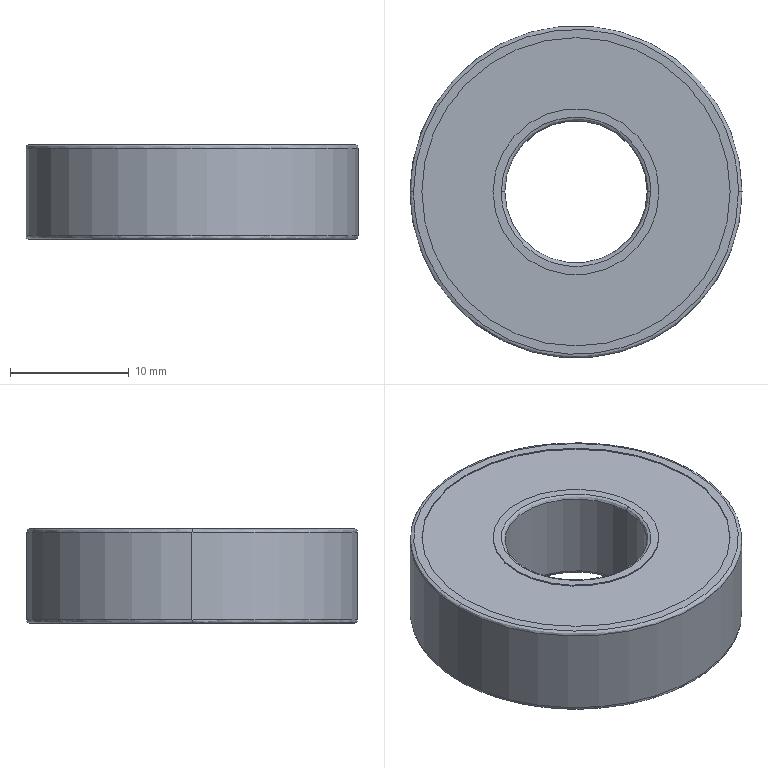Part | SolidWorks | features BaseBody 1 | 1 solid | 26 faces | box 28 x 28 x 8 mm | volume 3942 mm3 | cylinder 12 | spline 8 | plane 6 | commonest cylinder face diameters 14 x4 26 x4 12 x2 28 x2
STEP:
#1=CARTESIAN_POINT('',(-13.7,0.,-8.));
#2=VERTEX_POINT('',#1);
#3=CARTESIAN_POINT('',(13.7,0.,-8.));
#4=VERTEX_POINT('',#3);
#5=CARTESIAN_POINT('',(-13.7,0.,-8.));
#6=CARTESIAN_POINT('',(-13.7,-27.4,-8.));
#7=CARTESIAN_POINT('',(13.7,-27.4,-8.));
#8=CARTESIAN_POINT('',(13.7,0.,-8.));
#9=(BOUNDED_CURVE()B_SPLINE_CURVE(3,(#5,#6,#7,#8),.UNSPECIFIED.,.F.,.F.)B_SPLINE_CURVE_WITH_KNOTS((4,4),(0.,0.5),.UNSPECIFIED.)CURVE()GEOMETRIC_REPRESENTATION_ITEM()RATIONAL_B_SPLINE_CURVE((1.,0.3333,0.3333,1.))REPRESENTATION_ITEM(''));
#10=EDGE_CURVE('',#2,#4,#9,.T.);
#11=ORIENTED_EDGE('',*,*,#10,.T.);
#12=CARTESIAN_POINT('',(14.,0.,-7.7));
#13=VERTEX_POINT('',#12);
#14=CARTESIAN_POINT('',(13.7,0.,-7.7));
#15=DIRECTION('',(0.,-1.,0.));
#16=DIRECTION('',(1.,0.,0.));
#17=AXIS2_PLACEMENT_3D('',#14,#15,#16);
#18=CIRCLE('',#17,0.3);
#19=EDGE_CURVE('',#4,#13,#18,.T.);
#20=ORIENTED_EDGE('',*,*,#19,.T.);
#21=CARTESIAN_POINT('',(-14.,0.,-7.7));
#22=VERTEX_POINT('',#21);
#23=CARTESIAN_POINT('',(0.,0.,-7.7));
#24=DIRECTION('',(0.,0.,1.));
#25=DIRECTION('',(1.,0.,0.));
#26=AXIS2_PLACEMENT_3D('',#23,#24,#25);
#27=CIRCLE('',#26,14.);
#28=EDGE_CURVE('',#22,#13,#27,.T.);
#29=ORIENTED_EDGE('',*,*,#28,.F.);
#30=CARTESIAN_POINT('',(-13.7,0.,-7.7));
#31=DIRECTION('',(0.,1.,0.));
#32=DIRECTION('',(-1.,0.,0.));
#33=AXIS2_PLACEMENT_3D('',#30,#31,#32);
#34=CIRCLE('',#33,0.3);
#35=EDGE_CURVE('',#2,#22,#34,.T.);
#36=ORIENTED_EDGE('',*,*,#35,.F.);
#37=EDGE_LOOP('',(#11,#20,#29,#36));
#38=FACE_OUTER_BOUND('',#37,.T.);
#39=CARTESIAN_POINT('',(13.7,0.,-8.));
#40=CARTESIAN_POINT('',(13.7,-27.4,-8.));
#41=CARTESIAN_POINT('',(-13.7,-27.4,-8.));
#42=CARTESIAN_POINT('',(-13.7,0.,-8.));
#43=CARTESIAN_POINT('',(13.876,0.,-8.));
#44=CARTESIAN_POINT('',(13.876,-27.751,-8.));
#45=CARTESIAN_POINT('',(-13.876,-27.751,-8.));
#46=CARTESIAN_POINT('',(-13.876,0.,-8.));
#47=CARTESIAN_POINT('',(14.,0.,-7.876));
#48=CARTESIAN_POINT('',(14.,-28.,-7.876));
#49=CARTESIAN_POINT('',(-14.,-28.,-7.876));
#50=CARTESIAN_POINT('',(-14.,0.,-7.876));
#51=CARTESIAN_POINT('',(14.,0.,-7.7));
#52=CARTESIAN_POINT('',(14.,-28.,-7.7));
#53=CARTESIAN_POINT('',(-14.,-28.,-7.7));
#54=CARTESIAN_POINT('',(-14.,0.,-7.7));
#55=(BOUNDED_SURFACE()B_SPLINE_SURFACE(3,3,((#39,#40,#41,#42),(#43,#44,#45,#46),(#47,#48,#49,#50),(#51,#52,#53,#54)),.UNSPECIFIED.,.F.,.F.,.F.)B_SPLINE_SURFACE_WITH_KNOTS((4,4),(4,4),(0.,1.),(0.,1.),.UNSPECIFIED.)GEOMETRIC_REPRESENTATION_ITEM()RATIONAL_B_SPLINE_SURFACE(((1.,0.3333,0.3333,1.),(0.8047,0.2682,0.2682,0.8047),(0.8047,0.2682,0.2682,0.8047),(1.,0.3333,0.3333,1.)))REPRESENTATION_ITEM('')SURFACE());
#56=ADVANCED_FACE('',(#38),#55,.T.);
#57=CARTESIAN_POINT('',(14.,0.,-0.3));
#58=VERTEX_POINT('',#57);
#59=CARTESIAN_POINT('',(-14.,0.,-0.3));
#60=VERTEX_POINT('',#59);
#61=CARTESIAN_POINT('',(0.,0.,-0.3));
#62=DIRECTION('',(0.,0.,-1.));
#63=DIRECTION('',(1.,0.,0.));
#64=AXIS2_PLACEMENT_3D('',#61,#62,#63);
#65=CIRCLE('',#64,14.);
#66=EDGE_CURVE('',#58,#60,#65,.T.);
#67=ORIENTED_EDGE('',*,*,#66,.F.);
#68=CARTESIAN_POINT('',(13.7,0.,0.));
#69=VERTEX_POINT('',#68);
#70=CARTESIAN_POINT('',(13.7,0.,-0.3));
#71=DIRECTION('',(0.,-1.,0.));
#72=DIRECTION('',(1.,0.,0.));
#73=AXIS2_PLACEMENT_3D('',#70,#71,#72);
#74=CIRCLE('',#73,0.3);
#75=EDGE_CURVE('',#58,#69,#74,.T.);
#76=ORIENTED_EDGE('',*,*,#75,.T.);
#77=CARTESIAN_POINT('',(-13.7,0.,0.));
#78=VERTEX_POINT('',#77);
#79=CARTESIAN_POINT('',(13.7,0.,0.));
#80=CARTESIAN_POINT('',(13.7,-27.4,0.));
#81=CARTESIAN_POINT('',(-13.7,-27.4,0.));
#82=CARTESIAN_POINT('',(-13.7,0.,0.));
#83=(BOUNDED_CURVE()B_SPLINE_CURVE(3,(#79,#80,#81,#82),.UNSPECIFIED.,.F.,.F.)B_SPLINE_CURVE_WITH_KNOTS((4,4),(0.5,1.),.UNSPECIFIED.)CURVE()GEOMETRIC_REPRESENTATION_ITEM()RATIONAL_B_SPLINE_CURVE((1.,0.3333,0.3333,1.))REPRESENTATION_ITEM(''));
#84=EDGE_CURVE('',#69,#78,#83,.T.);
#85=ORIENTED_EDGE('',*,*,#84,.T.);
#86=CARTESIAN_POINT('',(-13.7,0.,-0.3));
#87=DIRECTION('',(0.,1.,0.));
#88=DIRECTION('',(-1.,0.,0.));
#89=AXIS2_PLACEMENT_3D('',#86,#87,#88);
#90=CIRCLE('',#89,0.3);
#91=EDGE_CURVE('',#60,#78,#90,.T.);
#92=ORIENTED_EDGE('',*,*,#91,.F.);
#93=EDGE_LOOP('',(#67,#76,#85,#92));
#94=FACE_OUTER_BOUND('',#93,.T.);
#95=CARTESIAN_POINT('',(14.,0.,-0.3));
#96=CARTESIAN_POINT('',(14.,-28.,-0.3));
#97=CARTESIAN_POINT('',(-14.,-28.,-0.3));
#98=CARTESIAN_POINT('',(-14.,0.,-0.3));
#99=CARTESIAN_POINT('',(14.,0.,-0.1243));
#100=CARTESIAN_POINT('',(14.,-28.,-0.1243));
#101=CARTESIAN_POINT('',(-14.,-28.,-0.1243));
#102=CARTESIAN_POINT('',(-14.,0.,-0.1243));
#103=CARTESIAN_POINT('',(13.876,0.,0.));
#104=CARTESIAN_POINT('',(13.876,-27.751,0.));
#105=CARTESIAN_POINT('',(-13.876,-27.751,0.));
#106=CARTESIAN_POINT('',(-13.876,0.,0.));
#107=CARTESIAN_POINT('',(13.7,0.,0.));
#108=CARTESIAN_POINT('',(13.7,-27.4,0.));
#109=CARTESIAN_POINT('',(-13.7,-27.4,0.));
#110=CARTESIAN_POINT('',(-13.7,0.,0.));
#111=(BOUNDED_SURFACE()B_SPLINE_SURFACE(3,3,((#95,#96,#97,#98),(#99,#100,#101,#102),(#103,#104,#105,#106),(#107,#108,#109,#110)),.UNSPECIFIED.,.F.,.F.,.F.)B_SPLINE_SURFACE_WITH_KNOTS((4,4),(4,4),(0.,1.),(0.,1.),.UNSPECIFIED.)GEOMETRIC_REPRESENTATION_ITEM()RATIONAL_B_SPLINE_SURFACE(((1.,0.3333,0.3333,1.),(0.8047,0.2682,0.2682,0.8047),(0.8047,0.2682,0.2682,0.8047),(1.,0.3333,0.3333,1.)))REPRESENTATION_ITEM('')SURFACE());
#112=ADVANCED_FACE('',(#94),#111,.T.);
#113=CARTESIAN_POINT('',(-6.,0.,-7.7));
#114=VERTEX_POINT('',#113);
#115=CARTESIAN_POINT('',(6.,0.,-7.7));
#116=VERTEX_POINT('',#115);
#117=CARTESIAN_POINT('',(0.,0.,-7.7));
#118=DIRECTION('',(0.,0.,1.));
#119=DIRECTION('',(-1.,0.,0.));
#120=AXIS2_PLACEMENT_3D('',#117,#118,#119);
#121=CIRCLE('',#120,6.);
#122=EDGE_CURVE('',#114,#116,#121,.T.);
#123=ORIENTED_EDGE('',*,*,#122,.T.);
#124=CARTESIAN_POINT('',(6.3,0.,-8.));
#125=VERTEX_POINT('',#124);
#126=CARTESIAN_POINT('',(6.3,0.,-7.7));
#127=DIRECTION('',(0.,-1.,0.));
#128=DIRECTION('',(1.,0.,0.));
#129=AXIS2_PLACEMENT_3D('',#126,#127,#128);
#130=CIRCLE('',#129,0.3);
#131=EDGE_CURVE('',#116,#125,#130,.T.);
#132=ORIENTED_EDGE('',*,*,#131,.T.);
#133=CARTESIAN_POINT('',(-6.3,0.,-8.));
#134=VERTEX_POINT('',#133);
#135=CARTESIAN_POINT('',(-6.3,0.,-8.));
#136=CARTESIAN_POINT('',(-6.3,-0.1926,-8.));
#137=CARTESIAN_POINT('',(-6.287,-0.4803,-8.));
#138=CARTESIAN_POINT('',(-6.249,-0.814,-8.));
#139=CARTESIAN_POINT('',(-6.224,-0.9804,-8.));
#140=CARTESIAN_POINT('',(-6.212,-1.052,-8.));
#141=CARTESIAN_POINT('',(-6.203,-1.099,-8.));
#142=CARTESIAN_POINT('',(-6.199,-1.121,-8.));
#143=CARTESIAN_POINT('',(-6.158,-1.347,-8.));
#144=CARTESIAN_POINT('',(-6.088,-1.644,-8.));
#145=CARTESIAN_POINT('',(-5.981,-1.984,-8.));
#146=CARTESIAN_POINT('',(-5.93,-2.128,-8.));
#147=CARTESIAN_POINT('',(-5.895,-2.224,-8.));
#148=CARTESIAN_POINT('',(-5.877,-2.27,-8.));
#149=CARTESIAN_POINT('',(-5.779,-2.517,-8.));
#150=CARTESIAN_POINT('',(-5.648,-2.806,-8.));
#151=CARTESIAN_POINT('',(-5.494,-3.085,-8.));
#152=CARTESIAN_POINT('',(-5.387,-3.268,-8.));
#153=CARTESIAN_POINT('',(-5.333,-3.356,-8.));
#154=CARTESIAN_POINT('',(-5.035,-3.811,-8.));
#155=CARTESIAN_POINT('',(-4.762,-4.147,-8.));
#156=CARTESIAN_POINT('',(-4.301,-4.608,-8.));
#157=CARTESIAN_POINT('',(-4.06,-4.826,-8.));
#158=CARTESIAN_POINT('',(-3.76,-5.057,-8.));
#159=CARTESIAN_POINT('',(-3.627,-5.151,-8.));
#160=CARTESIAN_POINT('',(-3.538,-5.213,-8.));
#161=CARTESIAN_POINT('',(-3.492,-5.244,-8.));
#162=CARTESIAN_POINT('',(-3.269,-5.389,-8.));
#163=CARTESIAN_POINT('',(-2.995,-5.55,-8.));
#164=CARTESIAN_POINT('',(-2.661,-5.712,-8.));
#165=CARTESIAN_POINT('',(-2.516,-5.776,-8.));
#166=CARTESIAN_POINT('',(-2.418,-5.818,-8.));
#167=CARTESIAN_POINT('',(-2.366,-5.839,-8.));
#168=CARTESIAN_POINT('',(-2.129,-5.933,-8.));
#169=CARTESIAN_POINT('',(-1.84,-6.031,-8.));
#170=CARTESIAN_POINT('',(-1.496,-6.121,-8.));
#171=CARTESIAN_POINT('',(-1.322,-6.16,-8.));
#172=CARTESIAN_POINT('',(-1.247,-6.175,-8.));
#173=CARTESIAN_POINT('',(-1.197,-6.185,-8.));
#174=CARTESIAN_POINT('',(-1.17,-6.19,-8.));
#175=CARTESIAN_POINT('',(-0.7678,-6.265,-8.));
#176=CARTESIAN_POINT('',(-0.385,-6.3,-8.));
#177=CARTESIAN_POINT('',(0.1925,-6.3,-8.));
#178=CARTESIAN_POINT('',(0.4802,-6.287,-8.));
#179=CARTESIAN_POINT('',(0.8139,-6.249,-8.));
#180=CARTESIAN_POINT('',(0.9803,-6.224,-8.));
#181=CARTESIAN_POINT('',(1.051,-6.212,-8.));
#182=CARTESIAN_POINT('',(1.099,-6.203,-8.));
#183=CARTESIAN_POINT('',(1.121,-6.199,-8.));
#184=CARTESIAN_POINT('',(1.347,-6.158,-8.));
#185=CARTESIAN_POINT('',(1.644,-6.088,-8.));
#186=CARTESIAN_POINT('',(1.984,-5.981,-8.));
#187=CARTESIAN_POINT('',(2.128,-5.93,-8.));
#188=CARTESIAN_POINT('',(2.224,-5.895,-8.));
#189=CARTESIAN_POINT('',(2.27,-5.877,-8.));
#190=CARTESIAN_POINT('',(2.517,-5.779,-8.));
#191=CARTESIAN_POINT('',(2.806,-5.648,-8.));
#192=CARTESIAN_POINT('',(3.085,-5.494,-8.));
#193=CARTESIAN_POINT('',(3.268,-5.387,-8.));
#194=CARTESIAN_POINT('',(3.356,-5.333,-8.));
#195=CARTESIAN_POINT('',(3.811,-5.035,-8.));
#196=CARTESIAN_POINT('',(4.147,-4.762,-8.));
#197=CARTESIAN_POINT('',(4.608,-4.301,-8.));
#198=CARTESIAN_POINT('',(4.826,-4.06,-8.));
#199=CARTESIAN_POINT('',(5.057,-3.76,-8.));
#200=CARTESIAN_POINT('',(5.151,-3.627,-8.));
#201=CARTESIAN_POINT('',(5.213,-3.538,-8.));
#202=CARTESIAN_POINT('',(5.244,-3.492,-8.));
#203=CARTESIAN_POINT('',(5.389,-3.269,-8.));
#204=CARTESIAN_POINT('',(5.55,-2.995,-8.));
#205=CARTESIAN_POINT('',(5.712,-2.661,-8.));
#206=CARTESIAN_POINT('',(5.776,-2.516,-8.));
#207=CARTESIAN_POINT('',(5.818,-2.418,-8.));
#208=CARTESIAN_POINT('',(5.839,-2.366,-8.));
#209=CARTESIAN_POINT('',(5.933,-2.129,-8.));
#210=CARTESIAN_POINT('',(6.031,-1.84,-8.));
#211=CARTESIAN_POINT('',(6.121,-1.496,-8.));
#212=CARTESIAN_POINT('',(6.16,-1.322,-8.));
#213=CARTESIAN_POINT('',(6.175,-1.247,-8.));
#214=CARTESIAN_POINT('',(6.185,-1.197,-8.));
#215=CARTESIAN_POINT('',(6.19,-1.17,-8.));
#216=CARTESIAN_POINT('',(6.265,-0.7678,-8.));
#217=CARTESIAN_POINT('',(6.3,-0.385,-8.));
#218=CARTESIAN_POINT('',(6.3,0.,-8.));
#219=B_SPLINE_CURVE_WITH_KNOTS('',3,(#135,#136,#137,#138,#139,#140,#141,#142,#143,#144,#145,#146,#147,#148,#149,#150,#151,#152,#153,#154,#155,#156,#157,#158,#159,#160,#161,#162,#163,#164,#165,#166,#167,#168,#169,#170,#171,#172,#173,#174,#175,#176,#177,#178,#179,#180,#181,#182,#183,#184,#185,#186,#187,#188,#189,#190,#191,#192,#193,#194,#195,#196,#197,#198,#199,#200,#201,#202,#203,#204,#205,#206,#207,#208,#209,#210,#211,#212,#213,#214,#215,#216,#217,#218),.UNSPECIFIED.,.F.,.F.,(4,1,1,1,2,2,1,1,2,2,1,2,2,2,1,1,2,2,1,1,2,2,1,1,1,2,2,2,1,1,1,2,2,1,1,2,2,1,2,2,2,1,1,2,2,1,1,2,2,1,1,1,2,2,4),(0.,0.01563,0.02344,0.02734,0.0293,0.03125,0.04688,0.05469,0.05859,0.0625,0.07813,0.08594,0.09375,0.125,0.1406,0.1484,0.1523,0.1563,0.1719,0.1797,0.1836,0.1875,0.2031,0.2109,0.2148,0.2168,0.2188,0.25,0.2656,0.2734,0.2773,0.2793,0.2813,0.2969,0.3047,0.3086,0.3125,0.3281,0.3359,0.3438,0.375,0.3906,0.3984,0.4023,0.4063,0.4219,0.4297,0.4336,0.4375,0.4531,0.4609,0.4648,0.4668,0.4688,0.5),.UNSPECIFIED.);
#220=EDGE_CURVE('',#134,#125,#219,.T.);
#221=ORIENTED_EDGE('',*,*,#220,.F.);
#222=CARTESIAN_POINT('',(-6.3,0.,-7.7));
#223=DIRECTION('',(0.,1.,0.));
#224=DIRECTION('',(-1.,0.,0.));
#225=AXIS2_PLACEMENT_3D('',#222,#223,#224);
#226=CIRCLE('',#225,0.3);
#227=EDGE_CURVE('',#114,#134,#226,.T.);
#228=ORIENTED_EDGE('',*,*,#227,.F.);
#229=EDGE_LOOP('',(#123,#132,#221,#228));
#230=FACE_OUTER_BOUND('',#229,.T.);
#231=CARTESIAN_POINT('',(6.,0.,-7.7));
#232=CARTESIAN_POINT('',(6.,-12.,-7.7));
#233=CARTESIAN_POINT('',(-6.,-12.,-7.7));
#234=CARTESIAN_POINT('',(-6.,0.,-7.7));
#235=CARTESIAN_POINT('',(6.,0.,-7.876));
#236=CARTESIAN_POINT('',(6.,-12.,-7.876));
#237=CARTESIAN_POINT('',(-6.,-12.,-7.876));
#238=CARTESIAN_POINT('',(-6.,0.,-7.876));
#239=CARTESIAN_POINT('',(6.124,0.,-8.));
#240=CARTESIAN_POINT('',(6.124,-12.249,-8.));
#241=CARTESIAN_POINT('',(-6.124,-12.249,-8.));
#242=CARTESIAN_POINT('',(-6.124,0.,-8.));
#243=CARTESIAN_POINT('',(6.3,0.,-8.));
#244=CARTESIAN_POINT('',(6.3,-12.6,-8.));
#245=CARTESIAN_POINT('',(-6.3,-12.6,-8.));
#246=CARTESIAN_POINT('',(-6.3,0.,-8.));
#247=(BOUNDED_SURFACE()B_SPLINE_SURFACE(3,3,((#231,#232,#233,#234),(#235,#236,#237,#238),(#239,#240,#241,#242),(#243,#244,#245,#246)),.UNSPECIFIED.,.F.,.F.,.F.)B_SPLINE_SURFACE_WITH_KNOTS((4,4),(4,4),(0.,1.),(0.,1.),.UNSPECIFIED.)GEOMETRIC_REPRESENTATION_ITEM()RATIONAL_B_SPLINE_SURFACE(((1.,0.3333,0.3333,1.),(0.8047,0.2682,0.2682,0.8047),(0.8047,0.2682,0.2682,0.8047),(1.,0.3333,0.3333,1.)))REPRESENTATION_ITEM('')SURFACE());
#248=ADVANCED_FACE('',(#230),#247,.T.);
#249=CARTESIAN_POINT('',(6.3,0.,0.));
#250=VERTEX_POINT('',#249);
#251=CARTESIAN_POINT('',(-6.3,0.,0.));
#252=VERTEX_POINT('',#251);
#253=CARTESIAN_POINT('',(6.3,0.,0.));
#254=CARTESIAN_POINT('',(6.3,-0.1925,0.));
#255=CARTESIAN_POINT('',(6.287,-0.4802,0.));
#256=CARTESIAN_POINT('',(6.249,-0.8139,0.));
#257=CARTESIAN_POINT('',(6.224,-0.9803,0.));
#258=CARTESIAN_POINT('',(6.212,-1.051,0.));
#259=CARTESIAN_POINT('',(6.203,-1.099,0.));
#260=CARTESIAN_POINT('',(6.199,-1.121,0.));
#261=CARTESIAN_POINT('',(6.158,-1.347,0.));
#262=CARTESIAN_POINT('',(6.088,-1.644,0.));
#263=CARTESIAN_POINT('',(5.981,-1.984,0.));
#264=CARTESIAN_POINT('',(5.93,-2.128,0.));
#265=CARTESIAN_POINT('',(5.895,-2.224,0.));
#266=CARTESIAN_POINT('',(5.877,-2.27,0.));
#267=CARTESIAN_POINT('',(5.779,-2.517,0.));
#268=CARTESIAN_POINT('',(5.648,-2.806,0.));
#269=CARTESIAN_POINT('',(5.494,-3.085,0.));
#270=CARTESIAN_POINT('',(5.387,-3.268,0.));
#271=CARTESIAN_POINT('',(5.333,-3.356,0.));
#272=CARTESIAN_POINT('',(5.035,-3.811,0.));
#273=CARTESIAN_POINT('',(4.762,-4.147,0.));
#274=CARTESIAN_POINT('',(4.301,-4.608,0.));
#275=CARTESIAN_POINT('',(4.06,-4.826,0.));
#276=CARTESIAN_POINT('',(3.76,-5.057,0.));
#277=CARTESIAN_POINT('',(3.627,-5.151,0.));
#278=CARTESIAN_POINT('',(3.538,-5.213,0.));
#279=CARTESIAN_POINT('',(3.492,-5.244,0.));
#280=CARTESIAN_POINT('',(3.269,-5.389,0.));
#281=CARTESIAN_POINT('',(2.995,-5.55,0.));
#282=CARTESIAN_POINT('',(2.661,-5.712,0.));
#283=CARTESIAN_POINT('',(2.516,-5.776,0.));
#284=CARTESIAN_POINT('',(2.418,-5.818,0.));
#285=CARTESIAN_POINT('',(2.366,-5.839,0.));
#286=CARTESIAN_POINT('',(2.129,-5.933,0.));
#287=CARTESIAN_POINT('',(1.84,-6.031,0.));
#288=CARTESIAN_POINT('',(1.496,-6.121,0.));
#289=CARTESIAN_POINT('',(1.322,-6.16,0.));
#290=CARTESIAN_POINT('',(1.247,-6.175,0.));
#291=CARTESIAN_POINT('',(1.197,-6.185,0.));
#292=CARTESIAN_POINT('',(1.17,-6.19,0.));
#293=CARTESIAN_POINT('',(0.7678,-6.265,0.));
#294=CARTESIAN_POINT('',(0.385,-6.3,0.));
#295=CARTESIAN_POINT('',(-0.1925,-6.3,0.));
#296=CARTESIAN_POINT('',(-0.4802,-6.287,0.));
#297=CARTESIAN_POINT('',(-0.8139,-6.249,0.));
#298=CARTESIAN_POINT('',(-0.9803,-6.224,0.));
#299=CARTESIAN_POINT('',(-1.051,-6.212,0.));
#300=CARTESIAN_POINT('',(-1.099,-6.203,0.));
#301=CARTESIAN_POINT('',(-1.121,-6.199,0.));
#302=CARTESIAN_POINT('',(-1.347,-6.158,0.));
#303=CARTESIAN_POINT('',(-1.644,-6.088,0.));
#304=CARTESIAN_POINT('',(-1.984,-5.981,0.));
#305=CARTESIAN_POINT('',(-2.128,-5.93,0.));
#306=CARTESIAN_POINT('',(-2.224,-5.895,0.));
#307=CARTESIAN_POINT('',(-2.27,-5.877,0.));
#308=CARTESIAN_POINT('',(-2.517,-5.779,0.));
#309=CARTESIAN_POINT('',(-2.806,-5.648,0.));
#310=CARTESIAN_POINT('',(-3.085,-5.494,0.));
#311=CARTESIAN_POINT('',(-3.268,-5.387,0.));
#312=CARTESIAN_POINT('',(-3.356,-5.333,0.));
#313=CARTESIAN_POINT('',(-3.811,-5.035,0.));
#314=CARTESIAN_POINT('',(-4.147,-4.762,0.));
#315=CARTESIAN_POINT('',(-4.608,-4.301,0.));
#316=CARTESIAN_POINT('',(-4.826,-4.06,0.));
#317=CARTESIAN_POINT('',(-5.057,-3.76,0.));
#318=CARTESIAN_POINT('',(-5.151,-3.627,0.));
#319=CARTESIAN_POINT('',(-5.213,-3.538,0.));
#320=CARTESIAN_POINT('',(-5.244,-3.492,0.));
#321=CARTESIAN_POINT('',(-5.389,-3.269,0.));
#322=CARTESIAN_POINT('',(-5.55,-2.995,0.));
#323=CARTESIAN_POINT('',(-5.712,-2.661,0.));
#324=CARTESIAN_POINT('',(-5.776,-2.516,0.));
#325=CARTESIAN_POINT('',(-5.818,-2.418,0.));
#326=CARTESIAN_POINT('',(-5.839,-2.366,0.));
#327=CARTESIAN_POINT('',(-5.933,-2.129,0.));
#328=CARTESIAN_POINT('',(-6.031,-1.84,0.));
#329=CARTESIAN_POINT('',(-6.121,-1.496,0.));
#330=CARTESIAN_POINT('',(-6.16,-1.322,0.));
#331=CARTESIAN_POINT('',(-6.175,-1.247,0.));
#332=CARTESIAN_POINT('',(-6.185,-1.197,0.));
#333=CARTESIAN_POINT('',(-6.19,-1.17,0.));
#334=CARTESIAN_POINT('',(-6.265,-0.7676,0.));
#335=CARTESIAN_POINT('',(-6.3,-0.3855,0.));
#336=CARTESIAN_POINT('',(-6.3,0.,0.));
#337=B_SPLINE_CURVE_WITH_KNOTS('',3,(#253,#254,#255,#256,#257,#258,#259,#260,#261,#262,#263,#264,#265,#266,#267,#268,#269,#270,#271,#272,#273,#274,#275,#276,#277,#278,#279,#280,#281,#282,#283,#284,#285,#286,#287,#288,#289,#290,#291,#292,#293,#294,#295,#296,#297,#298,#299,#300,#301,#302,#303,#304,#305,#306,#307,#308,#309,#310,#311,#312,#313,#314,#315,#316,#317,#318,#319,#320,#321,#322,#323,#324,#325,#326,#327,#328,#329,#330,#331,#332,#333,#334,#335,#336),.UNSPECIFIED.,.F.,.F.,(4,1,1,1,2,2,1,1,2,2,1,2,2,2,1,1,2,2,1,1,2,2,1,1,1,2,2,2,1,1,1,2,2,1,1,2,2,1,2,2,2,1,1,2,2,1,1,2,2,1,1,1,2,2,4),(0.5,0.5156,0.5234,0.5273,0.5293,0.5313,0.5469,0.5547,0.5586,0.5625,0.5781,0.5859,0.5938,0.625,0.6406,0.6484,0.6523,0.6563,0.6719,0.6797,0.6836,0.6875,0.7031,0.7109,0.7148,0.7168,0.7188,0.75,0.7656,0.7734,0.7773,0.7793,0.7813,0.7969,0.8047,0.8086,0.8125,0.8281,0.8359,0.8438,0.875,0.8906,0.8984,0.9023,0.9063,0.9219,0.9297,0.9336,0.9375,0.9531,0.9609,0.9648,0.9668,0.9688,1.),.UNSPECIFIED.);
#338=EDGE_CURVE('',#250,#252,#337,.T.);
#339=ORIENTED_EDGE('',*,*,#338,.F.);
#340=CARTESIAN_POINT('',(6.,0.,-0.3));
#341=VERTEX_POINT('',#340);
#342=CARTESIAN_POINT('',(6.3,0.,-0.3));
#343=DIRECTION('',(0.,-1.,0.));
#344=DIRECTION('',(1.,0.,0.));
#345=AXIS2_PLACEMENT_3D('',#342,#343,#344);
#346=CIRCLE('',#345,0.3);
#347=EDGE_CURVE('',#250,#341,#346,.T.);
#348=ORIENTED_EDGE('',*,*,#347,.T.);
#349=CARTESIAN_POINT('',(-6.,0.,-0.3));
#350=VERTEX_POINT('',#349);
#351=CARTESIAN_POINT('',(0.,0.,-0.3));
#352=DIRECTION('',(0.,0.,-1.));
#353=DIRECTION('',(-1.,0.,0.));
#354=AXIS2_PLACEMENT_3D('',#351,#352,#353);
#355=CIRCLE('',#354,6.);
#356=EDGE_CURVE('',#341,#350,#355,.T.);
#357=ORIENTED_EDGE('',*,*,#356,.T.);
#358=CARTESIAN_POINT('',(-6.3,0.,-0.3));
#359=DIRECTION('',(0.,1.,0.));
#360=DIRECTION('',(-1.,0.,0.));
#361=AXIS2_PLACEMENT_3D('',#358,#359,#360);
#362=CIRCLE('',#361,0.3);
#363=EDGE_CURVE('',#252,#350,#362,.T.);
#364=ORIENTED_EDGE('',*,*,#363,.F.);
#365=EDGE_LOOP('',(#339,#348,#357,#364));
#366=FACE_OUTER_BOUND('',#365,.T.);
#367=CARTESIAN_POINT('',(6.3,0.,0.));
#368=CARTESIAN_POINT('',(6.3,-12.6,0.));
#369=CARTESIAN_POINT('',(-6.3,-12.6,0.));
#370=CARTESIAN_POINT('',(-6.3,0.,0.));
#371=CARTESIAN_POINT('',(6.124,0.,0.));
#372=CARTESIAN_POINT('',(6.124,-12.249,0.));
#373=CARTESIAN_POINT('',(-6.124,-12.249,0.));
#374=CARTESIAN_POINT('',(-6.124,0.,0.));
#375=CARTESIAN_POINT('',(6.,0.,-0.1243));
#376=CARTESIAN_POINT('',(6.,-12.,-0.1243));
#377=CARTESIAN_POINT('',(-6.,-12.,-0.1243));
#378=CARTESIAN_POINT('',(-6.,0.,-0.1243));
#379=CARTESIAN_POINT('',(6.,0.,-0.3));
#380=CARTESIAN_POINT('',(6.,-12.,-0.3));
#381=CARTESIAN_POINT('',(-6.,-12.,-0.3));
#382=CARTESIAN_POINT('',(-6.,0.,-0.3));
#383=(BOUNDED_SURFACE()B_SPLINE_SURFACE(3,3,((#367,#368,#369,#370),(#371,#372,#373,#374),(#375,#376,#377,#378),(#379,#380,#381,#382)),.UNSPECIFIED.,.F.,.F.,.F.)B_SPLINE_SURFACE_WITH_KNOTS((4,4),(4,4),(0.,1.),(0.,1.),.UNSPECIFIED.)GEOMETRIC_REPRESENTATION_ITEM()RATIONAL_B_SPLINE_SURFACE(((1.,0.3333,0.3333,1.),(0.8047,0.2682,0.2682,0.8047),(0.8047,0.2682,0.2682,0.8047),(1.,0.3333,0.3333,1.)))REPRESENTATION_ITEM('')SURFACE());
#384=ADVANCED_FACE('',(#366),#383,.T.);
#385=CARTESIAN_POINT('',(0.,0.,-7.7));
#386=DIRECTION('',(0.,0.,1.));
#387=DIRECTION('',(1.,0.,0.));
#388=AXIS2_PLACEMENT_3D('',#385,#386,#387);
#389=CIRCLE('',#388,14.);
#390=EDGE_CURVE('',#13,#22,#389,.T.);
#391=ORIENTED_EDGE('',*,*,#390,.T.);
#392=CARTESIAN_POINT('',(-14.,0.,-8.));
#393=DIRECTION('',(0.,0.,1.));
#394=VECTOR('',#393,1000.);
#395=LINE('',#392,#394);
#396=EDGE_CURVE('',#22,#60,#395,.T.);
#397=ORIENTED_EDGE('',*,*,#396,.T.);
#398=CARTESIAN_POINT('',(0.,0.,-0.3));
#399=DIRECTION('',(0.,0.,-1.));
#400=DIRECTION('',(1.,0.,0.));
#401=AXIS2_PLACEMENT_3D('',#398,#399,#400);
#402=CIRCLE('',#401,14.);
#403=EDGE_CURVE('',#60,#58,#402,.T.);
#404=ORIENTED_EDGE('',*,*,#403,.T.);
#405=CARTESIAN_POINT('',(14.,0.,-8.));
#406=DIRECTION('',(0.,0.,1.));
#407=VECTOR('',#406,1000.);
#408=LINE('',#405,#407);
#409=EDGE_CURVE('',#13,#58,#408,.T.);
#410=ORIENTED_EDGE('',*,*,#409,.F.);
#411=EDGE_LOOP('',(#391,#397,#404,#410));
#412=FACE_OUTER_BOUND('',#411,.T.);
#413=CARTESIAN_POINT('',(0.,0.,-8.));
#414=DIRECTION('',(0.,0.,1.));
#415=DIRECTION('',(1.,0.,0.));
#416=AXIS2_PLACEMENT_3D('',#413,#414,#415);
#417=CYLINDRICAL_SURFACE('',#416,14.);
#418=ADVANCED_FACE('',(#412),#417,.T.);
#419=CARTESIAN_POINT('',(-13.,0.,-8.));
#420=VERTEX_POINT('',#419);
#421=CARTESIAN_POINT('',(13.,0.,-8.));
#422=VERTEX_POINT('',#421);
#423=CARTESIAN_POINT('',(0.,0.,-8.));
#424=DIRECTION('',(0.,0.,1.));
#425=DIRECTION('',(1.,0.,0.));
#426=AXIS2_PLACEMENT_3D('',#423,#424,#425);
#427=CIRCLE('',#426,13.);
#428=EDGE_CURVE('',#420,#422,#427,.T.);
#429=ORIENTED_EDGE('',*,*,#428,.F.);
#430=CARTESIAN_POINT('',(-13.,0.,-7.9));
#431=VERTEX_POINT('',#430);
#432=CARTESIAN_POINT('',(-13.,0.,-8.));
#433=DIRECTION('',(0.,0.,1.));
#434=VECTOR('',#433,1000.);
#435=LINE('',#432,#434);
#436=EDGE_CURVE('',#420,#431,#435,.T.);
#437=ORIENTED_EDGE('',*,*,#436,.T.);
#438=CARTESIAN_POINT('',(13.,0.,-7.9));
#439=VERTEX_POINT('',#438);
#440=CARTESIAN_POINT('',(0.,0.,-7.9));
#441=DIRECTION('',(0.,0.,-1.));
#442=DIRECTION('',(1.,0.,0.));
#443=AXIS2_PLACEMENT_3D('',#440,#441,#442);
#444=CIRCLE('',#443,13.);
#445=EDGE_CURVE('',#439,#431,#444,.T.);
#446=ORIENTED_EDGE('',*,*,#445,.F.);
#447=CARTESIAN_POINT('',(13.,0.,-8.));
#448=DIRECTION('',(0.,0.,1.));
#449=VECTOR('',#448,1000.);
#450=LINE('',#447,#449);
#451=EDGE_CURVE('',#422,#439,#450,.T.);
#452=ORIENTED_EDGE('',*,*,#451,.F.);
#453=EDGE_LOOP('',(#429,#437,#446,#452));
#454=FACE_OUTER_BOUND('',#453,.T.);
#455=CARTESIAN_POINT('',(0.,0.,-8.));
#456=DIRECTION('',(0.,0.,1.));
#457=DIRECTION('',(1.,0.,0.));
#458=AXIS2_PLACEMENT_3D('',#455,#456,#457);
#459=CYLINDRICAL_SURFACE('',#458,13.);
#460=ADVANCED_FACE('',(#454),#459,.F.);
#461=CARTESIAN_POINT('',(-13.,0.,-0.1));
#462=VERTEX_POINT('',#461);
#463=CARTESIAN_POINT('',(13.,0.,-0.1));
#464=VERTEX_POINT('',#463);
#465=CARTESIAN_POINT('',(0.,0.,-0.1));
#466=DIRECTION('',(0.,0.,1.));
#467=DIRECTION('',(1.,0.,0.));
#468=AXIS2_PLACEMENT_3D('',#465,#466,#467);
#469=CIRCLE('',#468,13.);
#470=EDGE_CURVE('',#462,#464,#469,.T.);
#471=ORIENTED_EDGE('',*,*,#470,.F.);
#472=CARTESIAN_POINT('',(-13.,0.,0.));
#473=VERTEX_POINT('',#472);
#474=CARTESIAN_POINT('',(-13.,0.,-8.));
#475=DIRECTION('',(0.,0.,1.));
#476=VECTOR('',#475,1000.);
#477=LINE('',#474,#476);
#478=EDGE_CURVE('',#462,#473,#477,.T.);
#479=ORIENTED_EDGE('',*,*,#478,.T.);
#480=CARTESIAN_POINT('',(13.,0.,0.));
#481=VERTEX_POINT('',#480);
#482=CARTESIAN_POINT('',(0.,0.,0.));
#483=DIRECTION('',(0.,0.,-1.));
#484=DIRECTION('',(1.,0.,0.));
#485=AXIS2_PLACEMENT_3D('',#482,#483,#484);
#486=CIRCLE('',#485,13.);
#487=EDGE_CURVE('',#481,#473,#486,.T.);
#488=ORIENTED_EDGE('',*,*,#487,.F.);
#489=CARTESIAN_POINT('',(13.,0.,-8.));
#490=DIRECTION('',(0.,0.,1.));
#491=VECTOR('',#490,1000.);
#492=LINE('',#489,#491);
#493=EDGE_CURVE('',#464,#481,#492,.T.);
#494=ORIENTED_EDGE('',*,*,#493,.F.);
#495=EDGE_LOOP('',(#471,#479,#488,#494));
#496=FACE_OUTER_BOUND('',#495,.T.);
#497=CARTESIAN_POINT('',(0.,0.,-8.));
#498=DIRECTION('',(0.,0.,1.));
#499=DIRECTION('',(1.,0.,0.));
#500=AXIS2_PLACEMENT_3D('',#497,#498,#499);
#501=CYLINDRICAL_SURFACE('',#500,13.);
#502=ADVANCED_FACE('',(#496),#501,.F.);
#503=CARTESIAN_POINT('',(7.,0.,-8.));
#504=VERTEX_POINT('',#503);
#505=CARTESIAN_POINT('',(-7.,0.,-8.));
#506=VERTEX_POINT('',#505);
#507=CARTESIAN_POINT('',(0.,0.,-8.));
#508=DIRECTION('',(0.,0.,1.));
#509=DIRECTION('',(1.,0.,0.));
#510=AXIS2_PLACEMENT_3D('',#507,#508,#509);
#511=CIRCLE('',#510,7.);
#512=EDGE_CURVE('',#504,#506,#511,.T.);
#513=ORIENTED_EDGE('',*,*,#512,.T.);
#514=CARTESIAN_POINT('',(-7.,0.,-7.9));
#515=VERTEX_POINT('',#514);
#516=CARTESIAN_POINT('',(-7.,0.,-8.));
#517=DIRECTION('',(0.,0.,1.));
#518=VECTOR('',#517,1000.);
#519=LINE('',#516,#518);
#520=EDGE_CURVE('',#506,#515,#519,.T.);
#521=ORIENTED_EDGE('',*,*,#520,.T.);
#522=CARTESIAN_POINT('',(7.,0.,-7.9));
#523=VERTEX_POINT('',#522);
#524=CARTESIAN_POINT('',(0.,0.,-7.9));
#525=DIRECTION('',(0.,0.,1.));
#526=DIRECTION('',(1.,0.,0.));
#527=AXIS2_PLACEMENT_3D('',#524,#525,#526);
#528=CIRCLE('',#527,7.);
#529=EDGE_CURVE('',#523,#515,#528,.T.);
#530=ORIENTED_EDGE('',*,*,#529,.F.);
#531=CARTESIAN_POINT('',(7.,0.,-8.));
#532=DIRECTION('',(0.,0.,1.));
#533=VECTOR('',#532,1000.);
#534=LINE('',#531,#533);
#535=EDGE_CURVE('',#504,#523,#534,.T.);
#536=ORIENTED_EDGE('',*,*,#535,.F.);
#537=EDGE_LOOP('',(#513,#521,#530,#536));
#538=FACE_OUTER_BOUND('',#537,.T.);
#539=CARTESIAN_POINT('',(0.,0.,-8.));
#540=DIRECTION('',(0.,0.,1.));
#541=DIRECTION('',(1.,0.,0.));
#542=AXIS2_PLACEMENT_3D('',#539,#540,#541);
#543=CYLINDRICAL_SURFACE('',#542,7.);
#544=ADVANCED_FACE('',(#538),#543,.T.);
#545=CARTESIAN_POINT('',(-7.,0.,-0.1));
#546=VERTEX_POINT('',#545);
#547=CARTESIAN_POINT('',(7.,0.,-0.1));
#548=VERTEX_POINT('',#547);
#549=CARTESIAN_POINT('',(0.,0.,-0.1));
#550=DIRECTION('',(0.,0.,-1.));
#551=DIRECTION('',(1.,0.,0.));
#552=AXIS2_PLACEMENT_3D('',#549,#550,#551);
#553=CIRCLE('',#552,7.);
#554=EDGE_CURVE('',#546,#548,#553,.T.);
#555=ORIENTED_EDGE('',*,*,#554,.F.);
#556=CARTESIAN_POINT('',(-7.,0.,0.));
#557=VERTEX_POINT('',#556);
#558=CARTESIAN_POINT('',(-7.,0.,-8.));
#559=DIRECTION('',(0.,0.,1.));
#560=VECTOR('',#559,1000.);
#561=LINE('',#558,#560);
#562=EDGE_CURVE('',#546,#557,#561,.T.);
#563=ORIENTED_EDGE('',*,*,#562,.T.);
#564=CARTESIAN_POINT('',(7.,0.,0.));
#565=VERTEX_POINT('',#564);
#566=CARTESIAN_POINT('',(0.,0.,0.));
#567=DIRECTION('',(0.,0.,-1.));
#568=DIRECTION('',(1.,0.,0.));
#569=AXIS2_PLACEMENT_3D('',#566,#567,#568);
#570=CIRCLE('',#569,7.);
#571=EDGE_CURVE('',#557,#565,#570,.T.);
#572=ORIENTED_EDGE('',*,*,#571,.T.);
#573=CARTESIAN_POINT('',(7.,0.,-8.));
#574=DIRECTION('',(0.,0.,1.));
#575=VECTOR('',#574,1000.);
#576=LINE('',#573,#575);
#577=EDGE_CURVE('',#548,#565,#576,.T.);
#578=ORIENTED_EDGE('',*,*,#577,.F.);
#579=EDGE_LOOP('',(#555,#563,#572,#578));
#580=FACE_OUTER_BOUND('',#579,.T.);
#581=CARTESIAN_POINT('',(0.,0.,-8.));
#582=DIRECTION('',(0.,0.,1.));
#583=DIRECTION('',(1.,0.,0.));
#584=AXIS2_PLACEMENT_3D('',#581,#582,#583);
#585=CYLINDRICAL_SURFACE('',#584,7.);
#586=ADVANCED_FACE('',(#580),#585,.T.);
#587=ORIENTED_EDGE('',*,*,#122,.F.);
#588=CARTESIAN_POINT('',(-6.,0.,-8.));
#589=DIRECTION('',(0.,0.,1.));
#590=VECTOR('',#589,1000.);
#591=LINE('',#588,#590);
#592=EDGE_CURVE('',#114,#350,#591,.T.);
#593=ORIENTED_EDGE('',*,*,#592,.T.);
#594=ORIENTED_EDGE('',*,*,#356,.F.);
#595=CARTESIAN_POINT('',(6.,0.,-8.));
#596=DIRECTION('',(0.,0.,1.));
#597=VECTOR('',#596,1000.);
#598=LINE('',#595,#597);
#599=EDGE_CURVE('',#116,#341,#598,.T.);
#600=ORIENTED_EDGE('',*,*,#599,.F.);
#601=EDGE_LOOP('',(#587,#593,#594,#600));
#602=FACE_OUTER_BOUND('',#601,.T.);
#603=CARTESIAN_POINT('',(0.,0.,-8.));
#604=DIRECTION('',(0.,0.,1.));
#605=DIRECTION('',(1.,0.,0.));
#606=AXIS2_PLACEMENT_3D('',#603,#604,#605);
#607=CYLINDRICAL_SURFACE('',#606,6.);
#608=ADVANCED_FACE('',(#602),#607,.F.);
#609=ORIENTED_EDGE('',*,*,#396,.F.);
#610=ORIENTED_EDGE('',*,*,#28,.T.);
#611=ORIENTED_EDGE('',*,*,#409,.T.);
#612=ORIENTED_EDGE('',*,*,#66,.T.);
#613=EDGE_LOOP('',(#609,#610,#611,#612));
#614=FACE_OUTER_BOUND('',#613,.T.);
#615=CARTESIAN_POINT('',(0.,0.,-8.));
#616=DIRECTION('',(0.,0.,1.));
#617=DIRECTION('',(1.,0.,0.));
#618=AXIS2_PLACEMENT_3D('',#615,#616,#617);
#619=CYLINDRICAL_SURFACE('',#618,14.);
#620=ADVANCED_FACE('',(#614),#619,.T.);
#621=ORIENTED_EDGE('',*,*,#19,.F.);
#622=CARTESIAN_POINT('',(13.7,0.,-8.));
#623=CARTESIAN_POINT('',(13.7,27.4,-8.));
#624=CARTESIAN_POINT('',(-13.7,27.4,-8.));
#625=CARTESIAN_POINT('',(-13.7,0.,-8.));
#626=(BOUNDED_CURVE()B_SPLINE_CURVE(3,(#622,#623,#624,#625),.UNSPECIFIED.,.F.,.F.)B_SPLINE_CURVE_WITH_KNOTS((4,4),(0.5,1.),.UNSPECIFIED.)CURVE()GEOMETRIC_REPRESENTATION_ITEM()RATIONAL_B_SPLINE_CURVE((1.,0.3333,0.3333,1.))REPRESENTATION_ITEM(''));
#627=EDGE_CURVE('',#4,#2,#626,.T.);
#628=ORIENTED_EDGE('',*,*,#627,.T.);
#629=ORIENTED_EDGE('',*,*,#35,.T.);
#630=ORIENTED_EDGE('',*,*,#390,.F.);
#631=EDGE_LOOP('',(#621,#628,#629,#630));
#632=FACE_OUTER_BOUND('',#631,.T.);
#633=CARTESIAN_POINT('',(-13.7,0.,-8.));
#634=CARTESIAN_POINT('',(-13.7,27.4,-8.));
#635=CARTESIAN_POINT('',(13.7,27.4,-8.));
#636=CARTESIAN_POINT('',(13.7,0.,-8.));
#637=CARTESIAN_POINT('',(-13.876,0.,-8.));
#638=CARTESIAN_POINT('',(-13.876,27.751,-8.));
#639=CARTESIAN_POINT('',(13.876,27.751,-8.));
#640=CARTESIAN_POINT('',(13.876,0.,-8.));
#641=CARTESIAN_POINT('',(-14.,0.,-7.876));
#642=CARTESIAN_POINT('',(-14.,28.,-7.876));
#643=CARTESIAN_POINT('',(14.,28.,-7.876));
#644=CARTESIAN_POINT('',(14.,0.,-7.876));
#645=CARTESIAN_POINT('',(-14.,0.,-7.7));
#646=CARTESIAN_POINT('',(-14.,28.,-7.7));
#647=CARTESIAN_POINT('',(14.,28.,-7.7));
#648=CARTESIAN_POINT('',(14.,0.,-7.7));
#649=(BOUNDED_SURFACE()B_SPLINE_SURFACE(3,3,((#633,#634,#635,#636),(#637,#638,#639,#640),(#641,#642,#643,#644),(#645,#646,#647,#648)),.UNSPECIFIED.,.F.,.F.,.F.)B_SPLINE_SURFACE_WITH_KNOTS((4,4),(4,4),(0.,1.),(0.,1.),.UNSPECIFIED.)GEOMETRIC_REPRESENTATION_ITEM()RATIONAL_B_SPLINE_SURFACE(((1.,0.3333,0.3333,1.),(0.8047,0.2682,0.2682,0.8047),(0.8047,0.2682,0.2682,0.8047),(1.,0.3333,0.3333,1.)))REPRESENTATION_ITEM('')SURFACE());
#650=ADVANCED_FACE('',(#632),#649,.T.);
#651=ORIENTED_EDGE('',*,*,#75,.F.);
#652=ORIENTED_EDGE('',*,*,#403,.F.);
#653=ORIENTED_EDGE('',*,*,#91,.T.);
#654=CARTESIAN_POINT('',(-13.7,0.,0.));
#655=CARTESIAN_POINT('',(-13.7,27.4,0.));
#656=CARTESIAN_POINT('',(13.7,27.4,0.));
#657=CARTESIAN_POINT('',(13.7,0.,0.));
#658=(BOUNDED_CURVE()B_SPLINE_CURVE(3,(#654,#655,#656,#657),.UNSPECIFIED.,.F.,.F.)B_SPLINE_CURVE_WITH_KNOTS((4,4),(0.,0.5),.UNSPECIFIED.)CURVE()GEOMETRIC_REPRESENTATION_ITEM()RATIONAL_B_SPLINE_CURVE((1.,0.3333,0.3333,1.))REPRESENTATION_ITEM(''));
#659=EDGE_CURVE('',#78,#69,#658,.T.);
#660=ORIENTED_EDGE('',*,*,#659,.T.);
#661=EDGE_LOOP('',(#651,#652,#653,#660));
#662=FACE_OUTER_BOUND('',#661,.T.);
#663=CARTESIAN_POINT('',(-14.,0.,-0.3));
#664=CARTESIAN_POINT('',(-14.,28.,-0.3));
#665=CARTESIAN_POINT('',(14.,28.,-0.3));
#666=CARTESIAN_POINT('',(14.,0.,-0.3));
#667=CARTESIAN_POINT('',(-14.,0.,-0.1243));
#668=CARTESIAN_POINT('',(-14.,28.,-0.1243));
#669=CARTESIAN_POINT('',(14.,28.,-0.1243));
#670=CARTESIAN_POINT('',(14.,0.,-0.1243));
#671=CARTESIAN_POINT('',(-13.876,0.,0.));
#672=CARTESIAN_POINT('',(-13.876,27.751,0.));
#673=CARTESIAN_POINT('',(13.876,27.751,0.));
#674=CARTESIAN_POINT('',(13.876,0.,0.));
#675=CARTESIAN_POINT('',(-13.7,0.,0.));
#676=CARTESIAN_POINT('',(-13.7,27.4,0.));
#677=CARTESIAN_POINT('',(13.7,27.4,0.));
#678=CARTESIAN_POINT('',(13.7,0.,0.));
#679=(BOUNDED_SURFACE()B_SPLINE_SURFACE(3,3,((#663,#664,#665,#666),(#667,#668,#669,#670),(#671,#672,#673,#674),(#675,#676,#677,#678)),.UNSPECIFIED.,.F.,.F.,.F.)B_SPLINE_SURFACE_WITH_KNOTS((4,4),(4,4),(0.,1.),(0.,1.),.UNSPECIFIED.)GEOMETRIC_REPRESENTATION_ITEM()RATIONAL_B_SPLINE_SURFACE(((1.,0.3333,0.3333,1.),(0.8047,0.2682,0.2682,0.8047),(0.8047,0.2682,0.2682,0.8047),(1.,0.3333,0.3333,1.)))REPRESENTATION_ITEM('')SURFACE());
#680=ADVANCED_FACE('',(#662),#679,.T.);
#681=CARTESIAN_POINT('',(0.,0.,-8.));
#682=DIRECTION('',(0.,0.,1.));
#683=DIRECTION('',(1.,0.,0.));
#684=AXIS2_PLACEMENT_3D('',#681,#682,#683);
#685=CIRCLE('',#684,13.);
#686=EDGE_CURVE('',#422,#420,#685,.T.);
#687=ORIENTED_EDGE('',*,*,#686,.T.);
#688=ORIENTED_EDGE('',*,*,#428,.T.);
#689=EDGE_LOOP('',(#687,#688));
#690=FACE_BOUND('',#689,.T.);
#691=ORIENTED_EDGE('',*,*,#10,.F.);
#692=ORIENTED_EDGE('',*,*,#627,.F.);
#693=EDGE_LOOP('',(#691,#692));
#694=FACE_OUTER_BOUND('',#693,.T.);
#695=CARTESIAN_POINT('',(0.,13.,-8.));
#696=DIRECTION('',(0.,0.,-1.));
#697=DIRECTION('',(-1.,0.,0.));
#698=AXIS2_PLACEMENT_3D('',#695,#696,#697);
#699=PLANE('',#698);
#700=ADVANCED_FACE('',(#690,#694),#699,.T.);
#701=ORIENTED_EDGE('',*,*,#659,.F.);
#702=ORIENTED_EDGE('',*,*,#84,.F.);
#703=EDGE_LOOP('',(#701,#702));
#704=FACE_OUTER_BOUND('',#703,.T.);
#705=ORIENTED_EDGE('',*,*,#487,.T.);
#706=CARTESIAN_POINT('',(0.,0.,0.));
#707=DIRECTION('',(0.,0.,-1.));
#708=DIRECTION('',(1.,0.,0.));
#709=AXIS2_PLACEMENT_3D('',#706,#707,#708);
#710=CIRCLE('',#709,13.);
#711=EDGE_CURVE('',#473,#481,#710,.T.);
#712=ORIENTED_EDGE('',*,*,#711,.T.);
#713=EDGE_LOOP('',(#705,#712));
#714=FACE_BOUND('',#713,.T.);
#715=CARTESIAN_POINT('',(0.,13.7,0.));
#716=DIRECTION('',(0.,0.,1.));
#717=DIRECTION('',(1.,0.,0.));
#718=AXIS2_PLACEMENT_3D('',#715,#716,#717);
#719=PLANE('',#718);
#720=ADVANCED_FACE('',(#704,#714),#719,.T.);
#721=ORIENTED_EDGE('',*,*,#436,.F.);
#722=ORIENTED_EDGE('',*,*,#686,.F.);
#723=ORIENTED_EDGE('',*,*,#451,.T.);
#724=CARTESIAN_POINT('',(0.,0.,-7.9));
#725=DIRECTION('',(0.,0.,-1.));
#726=DIRECTION('',(1.,0.,0.));
#727=AXIS2_PLACEMENT_3D('',#724,#725,#726);
#728=CIRCLE('',#727,13.);
#729=EDGE_CURVE('',#431,#439,#728,.T.);
#730=ORIENTED_EDGE('',*,*,#729,.F.);
#731=EDGE_LOOP('',(#721,#722,#723,#730));
#732=FACE_OUTER_BOUND('',#731,.T.);
#733=CARTESIAN_POINT('',(0.,0.,-8.));
#734=DIRECTION('',(0.,0.,1.));
#735=DIRECTION('',(1.,0.,0.));
#736=AXIS2_PLACEMENT_3D('',#733,#734,#735);
#737=CYLINDRICAL_SURFACE('',#736,13.);
#738=ADVANCED_FACE('',(#732),#737,.F.);
#739=ORIENTED_EDGE('',*,*,#478,.F.);
#740=CARTESIAN_POINT('',(0.,0.,-0.1));
#741=DIRECTION('',(0.,0.,1.));
#742=DIRECTION('',(1.,0.,0.));
#743=AXIS2_PLACEMENT_3D('',#740,#741,#742);
#744=CIRCLE('',#743,13.);
#745=EDGE_CURVE('',#464,#462,#744,.T.);
#746=ORIENTED_EDGE('',*,*,#745,.F.);
#747=ORIENTED_EDGE('',*,*,#493,.T.);
#748=ORIENTED_EDGE('',*,*,#711,.F.);
#749=EDGE_LOOP('',(#739,#746,#747,#748));
#750=FACE_OUTER_BOUND('',#749,.T.);
#751=CARTESIAN_POINT('',(0.,0.,-8.));
#752=DIRECTION('',(0.,0.,1.));
#753=DIRECTION('',(1.,0.,0.));
#754=AXIS2_PLACEMENT_3D('',#751,#752,#753);
#755=CYLINDRICAL_SURFACE('',#754,13.);
#756=ADVANCED_FACE('',(#750),#755,.F.);
#757=ORIENTED_EDGE('',*,*,#529,.T.);
#758=CARTESIAN_POINT('',(0.,0.,-7.9));
#759=DIRECTION('',(0.,0.,1.));
#760=DIRECTION('',(1.,0.,0.));
#761=AXIS2_PLACEMENT_3D('',#758,#759,#760);
#762=CIRCLE('',#761,7.);
#763=EDGE_CURVE('',#515,#523,#762,.T.);
#764=ORIENTED_EDGE('',*,*,#763,.T.);
#765=EDGE_LOOP('',(#757,#764));
#766=FACE_BOUND('',#765,.T.);
#767=ORIENTED_EDGE('',*,*,#445,.T.);
#768=ORIENTED_EDGE('',*,*,#729,.T.);
#769=EDGE_LOOP('',(#767,#768));
#770=FACE_OUTER_BOUND('',#769,.T.);
#771=CARTESIAN_POINT('',(0.,7.,-7.9));
#772=DIRECTION('',(0.,0.,-1.));
#773=DIRECTION('',(-1.,0.,0.));
#774=AXIS2_PLACEMENT_3D('',#771,#772,#773);
#775=PLANE('',#774);
#776=ADVANCED_FACE('',(#766,#770),#775,.T.);
#777=ORIENTED_EDGE('',*,*,#745,.T.);
#778=ORIENTED_EDGE('',*,*,#470,.T.);
#779=EDGE_LOOP('',(#777,#778));
#780=FACE_OUTER_BOUND('',#779,.T.);
#781=CARTESIAN_POINT('',(0.,0.,-0.1));
#782=DIRECTION('',(0.,0.,-1.));
#783=DIRECTION('',(1.,0.,0.));
#784=AXIS2_PLACEMENT_3D('',#781,#782,#783);
#785=CIRCLE('',#784,7.);
#786=EDGE_CURVE('',#548,#546,#785,.T.);
#787=ORIENTED_EDGE('',*,*,#786,.T.);
#788=ORIENTED_EDGE('',*,*,#554,.T.);
#789=EDGE_LOOP('',(#787,#788));
#790=FACE_BOUND('',#789,.T.);
#791=CARTESIAN_POINT('',(0.,13.,-0.1));
#792=DIRECTION('',(0.,0.,1.));
#793=DIRECTION('',(1.,0.,0.));
#794=AXIS2_PLACEMENT_3D('',#791,#792,#793);
#795=PLANE('',#794);
#796=ADVANCED_FACE('',(#780,#790),#795,.T.);
#797=ORIENTED_EDGE('',*,*,#520,.F.);
#798=CARTESIAN_POINT('',(0.,0.,-8.));
#799=DIRECTION('',(0.,0.,1.));
#800=DIRECTION('',(1.,0.,0.));
#801=AXIS2_PLACEMENT_3D('',#798,#799,#800);
#802=CIRCLE('',#801,7.);
#803=EDGE_CURVE('',#506,#504,#802,.T.);
#804=ORIENTED_EDGE('',*,*,#803,.T.);
#805=ORIENTED_EDGE('',*,*,#535,.T.);
#806=ORIENTED_EDGE('',*,*,#763,.F.);
#807=EDGE_LOOP('',(#797,#804,#805,#806));
#808=FACE_OUTER_BOUND('',#807,.T.);
#809=CARTESIAN_POINT('',(0.,0.,-8.));
#810=DIRECTION('',(0.,0.,1.));
#811=DIRECTION('',(1.,0.,0.));
#812=AXIS2_PLACEMENT_3D('',#809,#810,#811);
#813=CYLINDRICAL_SURFACE('',#812,7.);
#814=ADVANCED_FACE('',(#808),#813,.T.);
#815=ORIENTED_EDGE('',*,*,#562,.F.);
#816=ORIENTED_EDGE('',*,*,#786,.F.);
#817=ORIENTED_EDGE('',*,*,#577,.T.);
#818=CARTESIAN_POINT('',(0.,0.,0.));
#819=DIRECTION('',(0.,0.,-1.));
#820=DIRECTION('',(1.,0.,0.));
#821=AXIS2_PLACEMENT_3D('',#818,#819,#820);
#822=CIRCLE('',#821,7.);
#823=EDGE_CURVE('',#565,#557,#822,.T.);
#824=ORIENTED_EDGE('',*,*,#823,.T.);
#825=EDGE_LOOP('',(#815,#816,#817,#824));
#826=FACE_OUTER_BOUND('',#825,.T.);
#827=CARTESIAN_POINT('',(0.,0.,-8.));
#828=DIRECTION('',(0.,0.,1.));
#829=DIRECTION('',(1.,0.,0.));
#830=AXIS2_PLACEMENT_3D('',#827,#828,#829);
#831=CYLINDRICAL_SURFACE('',#830,7.);
#832=ADVANCED_FACE('',(#826),#831,.T.);
#833=ORIENTED_EDGE('',*,*,#220,.T.);
#834=CARTESIAN_POINT('',(6.3,0.,-8.));
#835=CARTESIAN_POINT('',(6.3,0.1925,-8.));
#836=CARTESIAN_POINT('',(6.287,0.4802,-8.));
#837=CARTESIAN_POINT('',(6.249,0.8139,-8.));
#838=CARTESIAN_POINT('',(6.224,0.9803,-8.));
#839=CARTESIAN_POINT('',(6.212,1.051,-8.));
#840=CARTESIAN_POINT('',(6.203,1.099,-8.));
#841=CARTESIAN_POINT('',(6.199,1.121,-8.));
#842=CARTESIAN_POINT('',(6.158,1.347,-8.));
#843=CARTESIAN_POINT('',(6.088,1.644,-8.));
#844=CARTESIAN_POINT('',(5.981,1.984,-8.));
#845=CARTESIAN_POINT('',(5.93,2.128,-8.));
#846=CARTESIAN_POINT('',(5.895,2.224,-8.));
#847=CARTESIAN_POINT('',(5.877,2.27,-8.));
#848=CARTESIAN_POINT('',(5.779,2.517,-8.));
#849=CARTESIAN_POINT('',(5.648,2.806,-8.));
#850=CARTESIAN_POINT('',(5.494,3.085,-8.));
#851=CARTESIAN_POINT('',(5.387,3.268,-8.));
#852=CARTESIAN_POINT('',(5.333,3.356,-8.));
#853=CARTESIAN_POINT('',(5.035,3.811,-8.));
#854=CARTESIAN_POINT('',(4.762,4.147,-8.));
#855=CARTESIAN_POINT('',(4.301,4.608,-8.));
#856=CARTESIAN_POINT('',(4.06,4.826,-8.));
#857=CARTESIAN_POINT('',(3.76,5.057,-8.));
#858=CARTESIAN_POINT('',(3.627,5.151,-8.));
#859=CARTESIAN_POINT('',(3.538,5.213,-8.));
#860=CARTESIAN_POINT('',(3.492,5.244,-8.));
#861=CARTESIAN_POINT('',(3.269,5.389,-8.));
#862=CARTESIAN_POINT('',(2.995,5.55,-8.));
#863=CARTESIAN_POINT('',(2.661,5.712,-8.));
#864=CARTESIAN_POINT('',(2.516,5.776,-8.));
#865=CARTESIAN_POINT('',(2.418,5.818,-8.));
#866=CARTESIAN_POINT('',(2.366,5.839,-8.));
#867=CARTESIAN_POINT('',(2.129,5.933,-8.));
#868=CARTESIAN_POINT('',(1.84,6.031,-8.));
#869=CARTESIAN_POINT('',(1.496,6.121,-8.));
#870=CARTESIAN_POINT('',(1.322,6.16,-8.));
#871=CARTESIAN_POINT('',(1.247,6.175,-8.));
#872=CARTESIAN_POINT('',(1.197,6.185,-8.));
#873=CARTESIAN_POINT('',(1.17,6.19,-8.));
#874=CARTESIAN_POINT('',(0.7678,6.265,-8.));
#875=CARTESIAN_POINT('',(0.385,6.3,-8.));
#876=CARTESIAN_POINT('',(-0.1925,6.3,-8.));
#877=CARTESIAN_POINT('',(-0.4802,6.287,-8.));
#878=CARTESIAN_POINT('',(-0.8139,6.249,-8.));
#879=CARTESIAN_POINT('',(-0.9803,6.224,-8.));
#880=CARTESIAN_POINT('',(-1.051,6.212,-8.));
#881=CARTESIAN_POINT('',(-1.099,6.203,-8.));
#882=CARTESIAN_POINT('',(-1.121,6.199,-8.));
#883=CARTESIAN_POINT('',(-1.347,6.158,-8.));
#884=CARTESIAN_POINT('',(-1.644,6.088,-8.));
#885=CARTESIAN_POINT('',(-1.984,5.981,-8.));
#886=CARTESIAN_POINT('',(-2.128,5.93,-8.));
#887=CARTESIAN_POINT('',(-2.224,5.895,-8.));
#888=CARTESIAN_POINT('',(-2.27,5.877,-8.));
#889=CARTESIAN_POINT('',(-2.517,5.779,-8.));
#890=CARTESIAN_POINT('',(-2.806,5.648,-8.));
#891=CARTESIAN_POINT('',(-3.085,5.494,-8.));
#892=CARTESIAN_POINT('',(-3.268,5.387,-8.));
#893=CARTESIAN_POINT('',(-3.356,5.333,-8.));
#894=CARTESIAN_POINT('',(-3.811,5.035,-8.));
#895=CARTESIAN_POINT('',(-4.147,4.762,-8.));
#896=CARTESIAN_POINT('',(-4.608,4.301,-8.));
#897=CARTESIAN_POINT('',(-4.826,4.06,-8.));
#898=CARTESIAN_POINT('',(-5.057,3.76,-8.));
#899=CARTESIAN_POINT('',(-5.151,3.627,-8.));
#900=CARTESIAN_POINT('',(-5.213,3.538,-8.));
#901=CARTESIAN_POINT('',(-5.244,3.492,-8.));
#902=CARTESIAN_POINT('',(-5.389,3.269,-8.));
#903=CARTESIAN_POINT('',(-5.55,2.995,-8.));
#904=CARTESIAN_POINT('',(-5.712,2.661,-8.));
#905=CARTESIAN_POINT('',(-5.776,2.516,-8.));
#906=CARTESIAN_POINT('',(-5.818,2.418,-8.));
#907=CARTESIAN_POINT('',(-5.839,2.366,-8.));
#908=CARTESIAN_POINT('',(-5.933,2.129,-8.));
#909=CARTESIAN_POINT('',(-6.031,1.84,-8.));
#910=CARTESIAN_POINT('',(-6.121,1.496,-8.));
#911=CARTESIAN_POINT('',(-6.16,1.322,-8.));
#912=CARTESIAN_POINT('',(-6.175,1.247,-8.));
#913=CARTESIAN_POINT('',(-6.185,1.197,-8.));
#914=CARTESIAN_POINT('',(-6.19,1.17,-8.));
#915=CARTESIAN_POINT('',(-6.265,0.7676,-8.));
#916=CARTESIAN_POINT('',(-6.3,0.3855,-8.));
#917=CARTESIAN_POINT('',(-6.3,0.,-8.));
#918=B_SPLINE_CURVE_WITH_KNOTS('',3,(#834,#835,#836,#837,#838,#839,#840,#841,#842,#843,#844,#845,#846,#847,#848,#849,#850,#851,#852,#853,#854,#855,#856,#857,#858,#859,#860,#861,#862,#863,#864,#865,#866,#867,#868,#869,#870,#871,#872,#873,#874,#875,#876,#877,#878,#879,#880,#881,#882,#883,#884,#885,#886,#887,#888,#889,#890,#891,#892,#893,#894,#895,#896,#897,#898,#899,#900,#901,#902,#903,#904,#905,#906,#907,#908,#909,#910,#911,#912,#913,#914,#915,#916,#917),.UNSPECIFIED.,.F.,.F.,(4,1,1,1,2,2,1,1,2,2,1,2,2,2,1,1,2,2,1,1,2,2,1,1,1,2,2,2,1,1,1,2,2,1,1,2,2,1,2,2,2,1,1,2,2,1,1,2,2,1,1,1,2,2,4),(0.5,0.5156,0.5234,0.5273,0.5293,0.5313,0.5469,0.5547,0.5586,0.5625,0.5781,0.5859,0.5938,0.625,0.6406,0.6484,0.6523,0.6563,0.6719,0.6797,0.6836,0.6875,0.7031,0.7109,0.7148,0.7168,0.7188,0.75,0.7656,0.7734,0.7773,0.7793,0.7813,0.7969,0.8047,0.8086,0.8125,0.8281,0.8359,0.8438,0.875,0.8906,0.8984,0.9023,0.9063,0.9219,0.9297,0.9336,0.9375,0.9531,0.9609,0.9648,0.9668,0.9688,1.),.UNSPECIFIED.);
#919=EDGE_CURVE('',#125,#134,#918,.T.);
#920=ORIENTED_EDGE('',*,*,#919,.T.);
#921=EDGE_LOOP('',(#833,#920));
#922=FACE_BOUND('',#921,.T.);
#923=ORIENTED_EDGE('',*,*,#512,.F.);
#924=ORIENTED_EDGE('',*,*,#803,.F.);
#925=EDGE_LOOP('',(#923,#924));
#926=FACE_OUTER_BOUND('',#925,.T.);
#927=CARTESIAN_POINT('',(0.,6.3,-8.));
#928=DIRECTION('',(0.,0.,-1.));
#929=DIRECTION('',(-1.,0.,0.));
#930=AXIS2_PLACEMENT_3D('',#927,#928,#929);
#931=PLANE('',#930);
#932=ADVANCED_FACE('',(#922,#926),#931,.T.);
#933=ORIENTED_EDGE('',*,*,#823,.F.);
#934=ORIENTED_EDGE('',*,*,#571,.F.);
#935=EDGE_LOOP('',(#933,#934));
#936=FACE_OUTER_BOUND('',#935,.T.);
#937=CARTESIAN_POINT('',(-6.3,0.,0.));
#938=CARTESIAN_POINT('',(-6.3,0.1926,0.));
#939=CARTESIAN_POINT('',(-6.287,0.4803,0.));
#940=CARTESIAN_POINT('',(-6.249,0.814,0.));
#941=CARTESIAN_POINT('',(-6.224,0.9804,0.));
#942=CARTESIAN_POINT('',(-6.212,1.052,0.));
#943=CARTESIAN_POINT('',(-6.203,1.099,0.));
#944=CARTESIAN_POINT('',(-6.199,1.121,0.));
#945=CARTESIAN_POINT('',(-6.158,1.347,0.));
#946=CARTESIAN_POINT('',(-6.088,1.644,0.));
#947=CARTESIAN_POINT('',(-5.981,1.984,0.));
#948=CARTESIAN_POINT('',(-5.93,2.128,0.));
#949=CARTESIAN_POINT('',(-5.895,2.224,0.));
#950=CARTESIAN_POINT('',(-5.877,2.27,0.));
#951=CARTESIAN_POINT('',(-5.779,2.517,0.));
#952=CARTESIAN_POINT('',(-5.648,2.806,0.));
#953=CARTESIAN_POINT('',(-5.494,3.085,0.));
#954=CARTESIAN_POINT('',(-5.387,3.268,0.));
#955=CARTESIAN_POINT('',(-5.333,3.356,0.));
#956=CARTESIAN_POINT('',(-5.035,3.811,0.));
#957=CARTESIAN_POINT('',(-4.762,4.147,0.));
#958=CARTESIAN_POINT('',(-4.301,4.608,0.));
#959=CARTESIAN_POINT('',(-4.06,4.826,0.));
#960=CARTESIAN_POINT('',(-3.76,5.057,0.));
#961=CARTESIAN_POINT('',(-3.627,5.151,0.));
#962=CARTESIAN_POINT('',(-3.538,5.213,0.));
#963=CARTESIAN_POINT('',(-3.492,5.244,0.));
#964=CARTESIAN_POINT('',(-3.269,5.389,0.));
#965=CARTESIAN_POINT('',(-2.995,5.55,0.));
#966=CARTESIAN_POINT('',(-2.661,5.712,0.));
#967=CARTESIAN_POINT('',(-2.516,5.776,0.));
#968=CARTESIAN_POINT('',(-2.418,5.818,0.));
#969=CARTESIAN_POINT('',(-2.366,5.839,0.));
#970=CARTESIAN_POINT('',(-2.129,5.933,0.));
#971=CARTESIAN_POINT('',(-1.84,6.031,0.));
#972=CARTESIAN_POINT('',(-1.496,6.121,0.));
#973=CARTESIAN_POINT('',(-1.322,6.16,0.));
#974=CARTESIAN_POINT('',(-1.247,6.175,0.));
#975=CARTESIAN_POINT('',(-1.197,6.185,0.));
#976=CARTESIAN_POINT('',(-1.17,6.19,0.));
#977=CARTESIAN_POINT('',(-0.7678,6.265,0.));
#978=CARTESIAN_POINT('',(-0.385,6.3,0.));
#979=CARTESIAN_POINT('',(0.1925,6.3,0.));
#980=CARTESIAN_POINT('',(0.4802,6.287,0.));
#981=CARTESIAN_POINT('',(0.8139,6.249,0.));
#982=CARTESIAN_POINT('',(0.9803,6.224,0.));
#983=CARTESIAN_POINT('',(1.051,6.212,0.));
#984=CARTESIAN_POINT('',(1.099,6.203,0.));
#985=CARTESIAN_POINT('',(1.121,6.199,0.));
#986=CARTESIAN_POINT('',(1.347,6.158,0.));
#987=CARTESIAN_POINT('',(1.644,6.088,0.));
#988=CARTESIAN_POINT('',(1.984,5.981,0.));
#989=CARTESIAN_POINT('',(2.128,5.93,0.));
#990=CARTESIAN_POINT('',(2.224,5.895,0.));
#991=CARTESIAN_POINT('',(2.27,5.877,0.));
#992=CARTESIAN_POINT('',(2.517,5.779,0.));
#993=CARTESIAN_POINT('',(2.806,5.648,0.));
#994=CARTESIAN_POINT('',(3.085,5.494,0.));
#995=CARTESIAN_POINT('',(3.268,5.387,0.));
#996=CARTESIAN_POINT('',(3.356,5.333,0.));
#997=CARTESIAN_POINT('',(3.811,5.035,0.));
#998=CARTESIAN_POINT('',(4.147,4.762,0.));
#999=CARTESIAN_POINT('',(4.608,4.301,0.));
#1000=CARTESIAN_POINT('',(4.826,4.06,0.));
#1001=CARTESIAN_POINT('',(5.057,3.76,0.));
#1002=CARTESIAN_POINT('',(5.151,3.627,0.));
#1003=CARTESIAN_POINT('',(5.213,3.538,0.));
#1004=CARTESIAN_POINT('',(5.244,3.492,0.));
#1005=CARTESIAN_POINT('',(5.389,3.269,0.));
#1006=CARTESIAN_POINT('',(5.55,2.995,0.));
#1007=CARTESIAN_POINT('',(5.712,2.661,0.));
#1008=CARTESIAN_POINT('',(5.776,2.516,0.));
#1009=CARTESIAN_POINT('',(5.818,2.418,0.));
#1010=CARTESIAN_POINT('',(5.839,2.366,0.));
#1011=CARTESIAN_POINT('',(5.933,2.129,0.));
#1012=CARTESIAN_POINT('',(6.031,1.84,0.));
#1013=CARTESIAN_POINT('',(6.121,1.496,0.));
#1014=CARTESIAN_POINT('',(6.16,1.322,0.));
#1015=CARTESIAN_POINT('',(6.175,1.247,0.));
#1016=CARTESIAN_POINT('',(6.185,1.197,0.));
#1017=CARTESIAN_POINT('',(6.19,1.17,0.));
#1018=CARTESIAN_POINT('',(6.265,0.7678,0.));
#1019=CARTESIAN_POINT('',(6.3,0.385,0.));
#1020=CARTESIAN_POINT('',(6.3,0.,0.));
#1021=B_SPLINE_CURVE_WITH_KNOTS('',3,(#937,#938,#939,#940,#941,#942,#943,#944,#945,#946,#947,#948,#949,#950,#951,#952,#953,#954,#955,#956,#957,#958,#959,#960,#961,#962,#963,#964,#965,#966,#967,#968,#969,#970,#971,#972,#973,#974,#975,#976,#977,#978,#979,#980,#981,#982,#983,#984,#985,#986,#987,#988,#989,#990,#991,#992,#993,#994,#995,#996,#997,#998,#999,#1000,#1001,#1002,#1003,#1004,#1005,#1006,#1007,#1008,#1009,#1010,#1011,#1012,#1013,#1014,#1015,#1016,#1017,#1018,#1019,#1020),.UNSPECIFIED.,.F.,.F.,(4,1,1,1,2,2,1,1,2,2,1,2,2,2,1,1,2,2,1,1,2,2,1,1,1,2,2,2,1,1,1,2,2,1,1,2,2,1,2,2,2,1,1,2,2,1,1,2,2,1,1,1,2,2,4),(0.,0.01563,0.02344,0.02734,0.0293,0.03125,0.04688,0.05469,0.05859,0.0625,0.07813,0.08594,0.09375,0.125,0.1406,0.1484,0.1523,0.1563,0.1719,0.1797,0.1836,0.1875,0.2031,0.2109,0.2148,0.2168,0.2188,0.25,0.2656,0.2734,0.2773,0.2793,0.2813,0.2969,0.3047,0.3086,0.3125,0.3281,0.3359,0.3438,0.375,0.3906,0.3984,0.4023,0.4063,0.4219,0.4297,0.4336,0.4375,0.4531,0.4609,0.4648,0.4668,0.4688,0.5),.UNSPECIFIED.);
#1022=EDGE_CURVE('',#252,#250,#1021,.T.);
#1023=ORIENTED_EDGE('',*,*,#1022,.T.);
#1024=ORIENTED_EDGE('',*,*,#338,.T.);
#1025=EDGE_LOOP('',(#1023,#1024));
#1026=FACE_BOUND('',#1025,.T.);
#1027=CARTESIAN_POINT('',(0.,7.,0.));
#1028=DIRECTION('',(0.,0.,1.));
#1029=DIRECTION('',(1.,0.,0.));
#1030=AXIS2_PLACEMENT_3D('',#1027,#1028,#1029);
#1031=PLANE('',#1030);
#1032=ADVANCED_FACE('',(#936,#1026),#1031,.T.);
#1033=ORIENTED_EDGE('',*,*,#131,.F.);
#1034=CARTESIAN_POINT('',(0.,0.,-7.7));
#1035=DIRECTION('',(0.,0.,1.));
#1036=DIRECTION('',(-1.,0.,0.));
#1037=AXIS2_PLACEMENT_3D('',#1034,#1035,#1036);
#1038=CIRCLE('',#1037,6.);
#1039=EDGE_CURVE('',#116,#114,#1038,.T.);
#1040=ORIENTED_EDGE('',*,*,#1039,.T.);
#1041=ORIENTED_EDGE('',*,*,#227,.T.);
#1042=ORIENTED_EDGE('',*,*,#919,.F.);
#1043=EDGE_LOOP('',(#1033,#1040,#1041,#1042));
#1044=FACE_OUTER_BOUND('',#1043,.T.);
#1045=CARTESIAN_POINT('',(-6.,0.,-7.7));
#1046=CARTESIAN_POINT('',(-6.,12.,-7.7));
#1047=CARTESIAN_POINT('',(6.,12.,-7.7));
#1048=CARTESIAN_POINT('',(6.,0.,-7.7));
#1049=CARTESIAN_POINT('',(-6.,0.,-7.876));
#1050=CARTESIAN_POINT('',(-6.,12.,-7.876));
#1051=CARTESIAN_POINT('',(6.,12.,-7.876));
#1052=CARTESIAN_POINT('',(6.,0.,-7.876));
#1053=CARTESIAN_POINT('',(-6.124,0.,-8.));
#1054=CARTESIAN_POINT('',(-6.124,12.249,-8.));
#1055=CARTESIAN_POINT('',(6.124,12.249,-8.));
#1056=CARTESIAN_POINT('',(6.124,0.,-8.));
#1057=CARTESIAN_POINT('',(-6.3,0.,-8.));
#1058=CARTESIAN_POINT('',(-6.3,12.6,-8.));
#1059=CARTESIAN_POINT('',(6.3,12.6,-8.));
#1060=CARTESIAN_POINT('',(6.3,0.,-8.));
#1061=(BOUNDED_SURFACE()B_SPLINE_SURFACE(3,3,((#1045,#1046,#1047,#1048),(#1049,#1050,#1051,#1052),(#1053,#1054,#1055,#1056),(#1057,#1058,#1059,#1060)),.UNSPECIFIED.,.F.,.F.,.F.)B_SPLINE_SURFACE_WITH_KNOTS((4,4),(4,4),(0.,1.),(0.,1.),.UNSPECIFIED.)GEOMETRIC_REPRESENTATION_ITEM()RATIONAL_B_SPLINE_SURFACE(((1.,0.3333,0.3333,1.),(0.8047,0.2682,0.2682,0.8047),(0.8047,0.2682,0.2682,0.8047),(1.,0.3333,0.3333,1.)))REPRESENTATION_ITEM('')SURFACE());
#1062=ADVANCED_FACE('',(#1044),#1061,.T.);
#1063=ORIENTED_EDGE('',*,*,#347,.F.);
#1064=ORIENTED_EDGE('',*,*,#1022,.F.);
#1065=ORIENTED_EDGE('',*,*,#363,.T.);
#1066=CARTESIAN_POINT('',(0.,0.,-0.3));
#1067=DIRECTION('',(0.,0.,-1.));
#1068=DIRECTION('',(-1.,0.,0.));
#1069=AXIS2_PLACEMENT_3D('',#1066,#1067,#1068);
#1070=CIRCLE('',#1069,6.);
#1071=EDGE_CURVE('',#350,#341,#1070,.T.);
#1072=ORIENTED_EDGE('',*,*,#1071,.T.);
#1073=EDGE_LOOP('',(#1063,#1064,#1065,#1072));
#1074=FACE_OUTER_BOUND('',#1073,.T.);
#1075=CARTESIAN_POINT('',(-6.3,0.,0.));
#1076=CARTESIAN_POINT('',(-6.3,12.6,0.));
#1077=CARTESIAN_POINT('',(6.3,12.6,0.));
#1078=CARTESIAN_POINT('',(6.3,0.,0.));
#1079=CARTESIAN_POINT('',(-6.124,0.,0.));
#1080=CARTESIAN_POINT('',(-6.124,12.249,0.));
#1081=CARTESIAN_POINT('',(6.124,12.249,0.));
#1082=CARTESIAN_POINT('',(6.124,0.,0.));
#1083=CARTESIAN_POINT('',(-6.,0.,-0.1243));
#1084=CARTESIAN_POINT('',(-6.,12.,-0.1243));
#1085=CARTESIAN_POINT('',(6.,12.,-0.1243));
#1086=CARTESIAN_POINT('',(6.,0.,-0.1243));
#1087=CARTESIAN_POINT('',(-6.,0.,-0.3));
#1088=CARTESIAN_POINT('',(-6.,12.,-0.3));
#1089=CARTESIAN_POINT('',(6.,12.,-0.3));
#1090=CARTESIAN_POINT('',(6.,0.,-0.3));
#1091=(BOUNDED_SURFACE()B_SPLINE_SURFACE(3,3,((#1075,#1076,#1077,#1078),(#1079,#1080,#1081,#1082),(#1083,#1084,#1085,#1086),(#1087,#1088,#1089,#1090)),.UNSPECIFIED.,.F.,.F.,.T.)B_SPLINE_SURFACE_WITH_KNOTS((4,4),(4,4),(0.,1.),(0.,1.),.UNSPECIFIED.)GEOMETRIC_REPRESENTATION_ITEM()RATIONAL_B_SPLINE_SURFACE(((1.,0.3333,0.3333,1.),(0.8047,0.2682,0.2682,0.8047),(0.8047,0.2682,0.2682,0.8047),(1.,0.3333,0.3333,1.)))REPRESENTATION_ITEM('')SURFACE());
#1092=ADVANCED_FACE('',(#1074),#1091,.T.);
#1093=ORIENTED_EDGE('',*,*,#592,.F.);
#1094=ORIENTED_EDGE('',*,*,#1039,.F.);
#1095=ORIENTED_EDGE('',*,*,#599,.T.);
#1096=ORIENTED_EDGE('',*,*,#1071,.F.);
#1097=EDGE_LOOP('',(#1093,#1094,#1095,#1096));
#1098=FACE_OUTER_BOUND('',#1097,.T.);
#1099=CARTESIAN_POINT('',(0.,0.,-8.));
#1100=DIRECTION('',(0.,0.,1.));
#1101=DIRECTION('',(1.,0.,0.));
#1102=AXIS2_PLACEMENT_3D('',#1099,#1100,#1101);
#1103=CYLINDRICAL_SURFACE('',#1102,6.);
#1104=ADVANCED_FACE('',(#1098),#1103,.F.);
#1105=CLOSED_SHELL('',(#56,#112,#248,#384,#418,#460,#502,#544,#586,#608,#620,#650,#680,#700,#720,#738,#756,#776,#796,#814,#832,#932,#1032,#1062,#1092,#1104));
#1106=MANIFOLD_SOLID_BREP('',#1105);
#1107=CARTESIAN_POINT('',(0.,0.,0.));
#1108=DIRECTION('',(0.,0.,1.));
#1109=DIRECTION('',(1.,0.,0.));
#1110=AXIS2_PLACEMENT_3D('',#1107,#1108,#1109);
#1111=(LENGTH_UNIT()NAMED_UNIT(*)SI_UNIT(.MILLI.,.METRE.));
#1112=UNCERTAINTY_MEASURE_WITH_UNIT(LENGTH_MEASURE(0.00001),#1111,'','');
#1113=(NAMED_UNIT(*)PLANE_ANGLE_UNIT()SI_UNIT($,.RADIAN.));
#1114=(NAMED_UNIT(*)SI_UNIT($,.STERADIAN.)SOLID_ANGLE_UNIT());
#1115=(GEOMETRIC_REPRESENTATION_CONTEXT(3)GLOBAL_UNCERTAINTY_ASSIGNED_CONTEXT((#1112))GLOBAL_UNIT_ASSIGNED_CONTEXT((#1111,#1113,#1114))REPRESENTATION_CONTEXT('',''));
#1116=ADVANCED_BREP_SHAPE_REPRESENTATION('',(#1106,#1110),#1115);